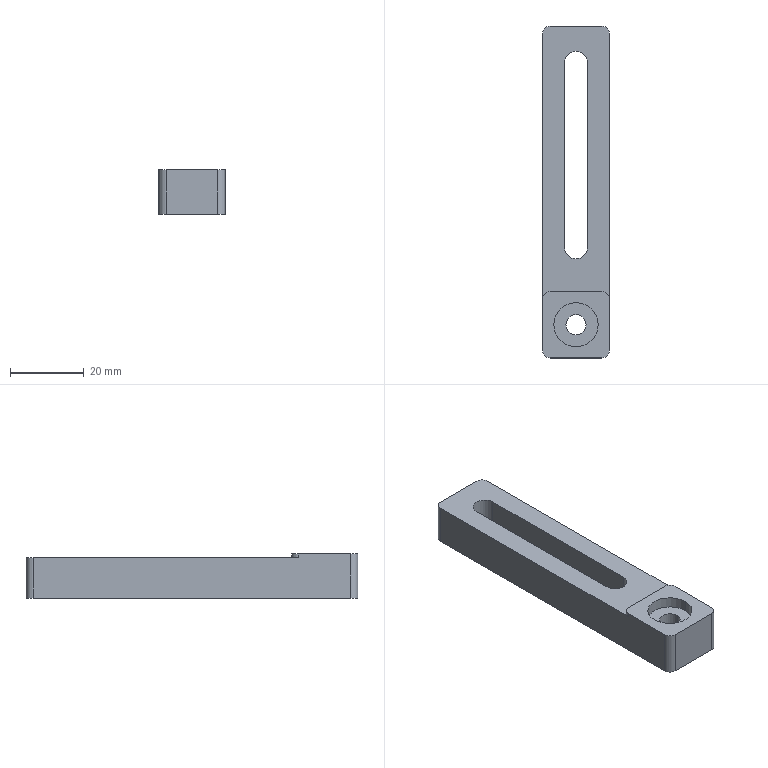Part | STEP file | 10000020588swp000-1 | 1 solid | 26 faces | box 18 x 90 x 12 mm | volume 13483 mm3 | cylinder 14 | plane 12 | commonest cylinder face diameters 4 x6 5.5 x2 6.3 x2 9.5 x2 12 x2
STEP:
#1=CARTESIAN_POINT('',(4.75,-36.,5.5));
#2=VERTEX_POINT('',#1);
#3=CARTESIAN_POINT('',(-4.75,-36.,5.5));
#4=VERTEX_POINT('',#3);
#5=CARTESIAN_POINT('',(0.,-36.,5.5));
#6=DIRECTION('',(0.,0.,-1.));
#7=DIRECTION('',(-1.,0.,0.));
#8=AXIS2_PLACEMENT_3D('',#5,#6,#7);
#9=CIRCLE('',#8,4.75);
#10=EDGE_CURVE('',#2,#4,#9,.T.);
#11=ORIENTED_EDGE('',*,*,#10,.F.);
#12=CARTESIAN_POINT('',(4.75,-36.,0.));
#13=VERTEX_POINT('',#12);
#14=CARTESIAN_POINT('',(4.75,-36.,0.));
#15=DIRECTION('',(0.,0.,-1.));
#16=VECTOR('',#15,1000.);
#17=LINE('',#14,#16);
#18=EDGE_CURVE('',#2,#13,#17,.T.);
#19=ORIENTED_EDGE('',*,*,#18,.T.);
#20=CARTESIAN_POINT('',(-4.75,-36.,0.));
#21=VERTEX_POINT('',#20);
#22=CARTESIAN_POINT('',(0.,-36.,0.));
#23=DIRECTION('',(0.,0.,-1.));
#24=DIRECTION('',(-1.,0.,0.));
#25=AXIS2_PLACEMENT_3D('',#22,#23,#24);
#26=CIRCLE('',#25,4.75);
#27=EDGE_CURVE('',#13,#21,#26,.T.);
#28=ORIENTED_EDGE('',*,*,#27,.T.);
#29=CARTESIAN_POINT('',(-4.75,-36.,0.));
#30=DIRECTION('',(0.,0.,-1.));
#31=VECTOR('',#30,1000.);
#32=LINE('',#29,#31);
#33=EDGE_CURVE('',#4,#21,#32,.T.);
#34=ORIENTED_EDGE('',*,*,#33,.F.);
#35=EDGE_LOOP('',(#11,#19,#28,#34));
#36=FACE_OUTER_BOUND('',#35,.T.);
#37=CARTESIAN_POINT('',(0.,-36.,0.));
#38=DIRECTION('',(0.,0.,-1.));
#39=DIRECTION('',(-1.,0.,0.));
#40=AXIS2_PLACEMENT_3D('',#37,#38,#39);
#41=CYLINDRICAL_SURFACE('',#40,4.75);
#42=ADVANCED_FACE('',(#36),#41,.F.);
#43=CARTESIAN_POINT('',(-6.,-36.,9.));
#44=VERTEX_POINT('',#43);
#45=CARTESIAN_POINT('',(6.,-36.,9.));
#46=VERTEX_POINT('',#45);
#47=CARTESIAN_POINT('',(0.,-36.,9.));
#48=DIRECTION('',(0.,0.,1.));
#49=DIRECTION('',(1.,0.,0.));
#50=AXIS2_PLACEMENT_3D('',#47,#48,#49);
#51=CIRCLE('',#50,6.);
#52=EDGE_CURVE('',#44,#46,#51,.T.);
#53=ORIENTED_EDGE('',*,*,#52,.F.);
#54=CARTESIAN_POINT('',(-6.,-36.,12.));
#55=VERTEX_POINT('',#54);
#56=CARTESIAN_POINT('',(-6.,-36.,12.));
#57=DIRECTION('',(0.,0.,1.));
#58=VECTOR('',#57,1000.);
#59=LINE('',#56,#58);
#60=EDGE_CURVE('',#44,#55,#59,.T.);
#61=ORIENTED_EDGE('',*,*,#60,.T.);
#62=CARTESIAN_POINT('',(6.,-36.,12.));
#63=VERTEX_POINT('',#62);
#64=CARTESIAN_POINT('',(0.,-36.,12.));
#65=DIRECTION('',(0.,0.,1.));
#66=DIRECTION('',(1.,0.,0.));
#67=AXIS2_PLACEMENT_3D('',#64,#65,#66);
#68=CIRCLE('',#67,6.);
#69=EDGE_CURVE('',#55,#63,#68,.T.);
#70=ORIENTED_EDGE('',*,*,#69,.T.);
#71=CARTESIAN_POINT('',(6.,-36.,12.));
#72=DIRECTION('',(0.,0.,1.));
#73=VECTOR('',#72,1000.);
#74=LINE('',#71,#73);
#75=EDGE_CURVE('',#46,#63,#74,.T.);
#76=ORIENTED_EDGE('',*,*,#75,.F.);
#77=EDGE_LOOP('',(#53,#61,#70,#76));
#78=FACE_OUTER_BOUND('',#77,.T.);
#79=CARTESIAN_POINT('',(0.,-36.,12.));
#80=DIRECTION('',(0.,0.,1.));
#81=DIRECTION('',(1.,0.,0.));
#82=AXIS2_PLACEMENT_3D('',#79,#80,#81);
#83=CYLINDRICAL_SURFACE('',#82,6.);
#84=ADVANCED_FACE('',(#78),#83,.F.);
#85=CARTESIAN_POINT('',(2.75,-36.,5.5));
#86=VERTEX_POINT('',#85);
#87=CARTESIAN_POINT('',(-2.75,-36.,5.5));
#88=VERTEX_POINT('',#87);
#89=CARTESIAN_POINT('',(0.,-36.,5.5));
#90=DIRECTION('',(0.,0.,-1.));
#91=DIRECTION('',(1.,0.,0.));
#92=AXIS2_PLACEMENT_3D('',#89,#90,#91);
#93=CIRCLE('',#92,2.75);
#94=EDGE_CURVE('',#86,#88,#93,.T.);
#95=ORIENTED_EDGE('',*,*,#94,.T.);
#96=CARTESIAN_POINT('',(-2.75,-36.,9.));
#97=VERTEX_POINT('',#96);
#98=CARTESIAN_POINT('',(-2.75,-36.,12.));
#99=DIRECTION('',(0.,0.,1.));
#100=VECTOR('',#99,1000.);
#101=LINE('',#98,#100);
#102=EDGE_CURVE('',#88,#97,#101,.T.);
#103=ORIENTED_EDGE('',*,*,#102,.T.);
#104=CARTESIAN_POINT('',(2.75,-36.,9.));
#105=VERTEX_POINT('',#104);
#106=CARTESIAN_POINT('',(0.,-36.,9.));
#107=DIRECTION('',(0.,0.,1.));
#108=DIRECTION('',(1.,0.,0.));
#109=AXIS2_PLACEMENT_3D('',#106,#107,#108);
#110=CIRCLE('',#109,2.75);
#111=EDGE_CURVE('',#97,#105,#110,.T.);
#112=ORIENTED_EDGE('',*,*,#111,.T.);
#113=CARTESIAN_POINT('',(2.75,-36.,12.));
#114=DIRECTION('',(0.,0.,1.));
#115=VECTOR('',#114,1000.);
#116=LINE('',#113,#115);
#117=EDGE_CURVE('',#86,#105,#116,.T.);
#118=ORIENTED_EDGE('',*,*,#117,.F.);
#119=EDGE_LOOP('',(#95,#103,#112,#118));
#120=FACE_OUTER_BOUND('',#119,.T.);
#121=CARTESIAN_POINT('',(0.,-36.,12.));
#122=DIRECTION('',(0.,0.,1.));
#123=DIRECTION('',(1.,0.,0.));
#124=AXIS2_PLACEMENT_3D('',#121,#122,#123);
#125=CYLINDRICAL_SURFACE('',#124,2.75);
#126=ADVANCED_FACE('',(#120),#125,.F.);
#127=CARTESIAN_POINT('',(7.,45.,0.));
#128=VERTEX_POINT('',#127);
#129=CARTESIAN_POINT('',(-7.,45.,0.));
#130=VERTEX_POINT('',#129);
#131=CARTESIAN_POINT('',(-9.,45.,0.));
#132=DIRECTION('',(-1.,0.,0.));
#133=VECTOR('',#132,1000.);
#134=LINE('',#131,#133);
#135=EDGE_CURVE('',#128,#130,#134,.T.);
#136=ORIENTED_EDGE('',*,*,#135,.T.);
#137=CARTESIAN_POINT('',(-7.,45.,11.));
#138=VERTEX_POINT('',#137);
#139=CARTESIAN_POINT('',(-7.,45.,12.));
#140=DIRECTION('',(0.,0.,1.));
#141=VECTOR('',#140,1000.);
#142=LINE('',#139,#141);
#143=EDGE_CURVE('',#130,#138,#142,.T.);
#144=ORIENTED_EDGE('',*,*,#143,.T.);
#145=CARTESIAN_POINT('',(7.,45.,11.));
#146=VERTEX_POINT('',#145);
#147=CARTESIAN_POINT('',(-9.,45.,11.));
#148=DIRECTION('',(-1.,0.,0.));
#149=VECTOR('',#148,1000.);
#150=LINE('',#147,#149);
#151=EDGE_CURVE('',#146,#138,#150,.T.);
#152=ORIENTED_EDGE('',*,*,#151,.F.);
#153=CARTESIAN_POINT('',(7.,45.,12.));
#154=DIRECTION('',(0.,0.,-1.));
#155=VECTOR('',#154,1000.);
#156=LINE('',#153,#155);
#157=EDGE_CURVE('',#146,#128,#156,.T.);
#158=ORIENTED_EDGE('',*,*,#157,.T.);
#159=EDGE_LOOP('',(#136,#144,#152,#158));
#160=FACE_OUTER_BOUND('',#159,.T.);
#161=CARTESIAN_POINT('',(-9.,45.,12.));
#162=DIRECTION('',(0.,-1.,0.));
#163=DIRECTION('',(0.,0.,-1.));
#164=AXIS2_PLACEMENT_3D('',#161,#162,#163);
#165=PLANE('',#164);
#166=ADVANCED_FACE('',(#160),#165,.F.);
#167=CARTESIAN_POINT('',(9.,-29.,11.));
#168=VERTEX_POINT('',#167);
#169=CARTESIAN_POINT('',(9.,43.,11.));
#170=VERTEX_POINT('',#169);
#171=CARTESIAN_POINT('',(9.,45.,11.));
#172=DIRECTION('',(0.,1.,0.));
#173=VECTOR('',#172,1000.);
#174=LINE('',#171,#173);
#175=EDGE_CURVE('',#168,#170,#174,.T.);
#176=ORIENTED_EDGE('',*,*,#175,.F.);
#177=CARTESIAN_POINT('',(9.,-29.,12.));
#178=VERTEX_POINT('',#177);
#179=CARTESIAN_POINT('',(9.,-29.,12.));
#180=DIRECTION('',(0.,0.,1.));
#181=VECTOR('',#180,1000.);
#182=LINE('',#179,#181);
#183=EDGE_CURVE('',#168,#178,#182,.T.);
#184=ORIENTED_EDGE('',*,*,#183,.T.);
#185=CARTESIAN_POINT('',(9.,-43.,12.));
#186=VERTEX_POINT('',#185);
#187=CARTESIAN_POINT('',(9.,45.,12.));
#188=DIRECTION('',(0.,1.,0.));
#189=VECTOR('',#188,1000.);
#190=LINE('',#187,#189);
#191=EDGE_CURVE('',#186,#178,#190,.T.);
#192=ORIENTED_EDGE('',*,*,#191,.F.);
#193=CARTESIAN_POINT('',(9.,-43.,0.));
#194=VERTEX_POINT('',#193);
#195=CARTESIAN_POINT('',(9.,-43.,12.));
#196=DIRECTION('',(0.,0.,-1.));
#197=VECTOR('',#196,1000.);
#198=LINE('',#195,#197);
#199=EDGE_CURVE('',#186,#194,#198,.T.);
#200=ORIENTED_EDGE('',*,*,#199,.T.);
#201=CARTESIAN_POINT('',(9.,43.,0.));
#202=VERTEX_POINT('',#201);
#203=CARTESIAN_POINT('',(9.,45.,0.));
#204=DIRECTION('',(0.,1.,0.));
#205=VECTOR('',#204,1000.);
#206=LINE('',#203,#205);
#207=EDGE_CURVE('',#194,#202,#206,.T.);
#208=ORIENTED_EDGE('',*,*,#207,.T.);
#209=CARTESIAN_POINT('',(9.,43.,12.));
#210=DIRECTION('',(0.,0.,1.));
#211=VECTOR('',#210,1000.);
#212=LINE('',#209,#211);
#213=EDGE_CURVE('',#202,#170,#212,.T.);
#214=ORIENTED_EDGE('',*,*,#213,.T.);
#215=EDGE_LOOP('',(#176,#184,#192,#200,#208,#214));
#216=FACE_OUTER_BOUND('',#215,.T.);
#217=CARTESIAN_POINT('',(9.,45.,12.));
#218=DIRECTION('',(-1.,0.,0.));
#219=DIRECTION('',(0.,-1.,0.));
#220=AXIS2_PLACEMENT_3D('',#217,#218,#219);
#221=PLANE('',#220);
#222=ADVANCED_FACE('',(#216),#221,.F.);
#223=CARTESIAN_POINT('',(-9.,-29.,12.));
#224=VERTEX_POINT('',#223);
#225=CARTESIAN_POINT('',(-9.,-43.,12.));
#226=VERTEX_POINT('',#225);
#227=CARTESIAN_POINT('',(-9.,45.,12.));
#228=DIRECTION('',(0.,-1.,0.));
#229=VECTOR('',#228,1000.);
#230=LINE('',#227,#229);
#231=EDGE_CURVE('',#224,#226,#230,.T.);
#232=ORIENTED_EDGE('',*,*,#231,.F.);
#233=CARTESIAN_POINT('',(-9.,-29.,11.));
#234=VERTEX_POINT('',#233);
#235=CARTESIAN_POINT('',(-9.,-29.,12.));
#236=DIRECTION('',(0.,0.,-1.));
#237=VECTOR('',#236,1000.);
#238=LINE('',#235,#237);
#239=EDGE_CURVE('',#224,#234,#238,.T.);
#240=ORIENTED_EDGE('',*,*,#239,.T.);
#241=CARTESIAN_POINT('',(-9.,43.,11.));
#242=VERTEX_POINT('',#241);
#243=CARTESIAN_POINT('',(-9.,45.,11.));
#244=DIRECTION('',(0.,-1.,0.));
#245=VECTOR('',#244,1000.);
#246=LINE('',#243,#245);
#247=EDGE_CURVE('',#242,#234,#246,.T.);
#248=ORIENTED_EDGE('',*,*,#247,.F.);
#249=CARTESIAN_POINT('',(-9.,43.,0.));
#250=VERTEX_POINT('',#249);
#251=CARTESIAN_POINT('',(-9.,43.,12.));
#252=DIRECTION('',(0.,0.,-1.));
#253=VECTOR('',#252,1000.);
#254=LINE('',#251,#253);
#255=EDGE_CURVE('',#242,#250,#254,.T.);
#256=ORIENTED_EDGE('',*,*,#255,.T.);
#257=CARTESIAN_POINT('',(-9.,-43.,0.));
#258=VERTEX_POINT('',#257);
#259=CARTESIAN_POINT('',(-9.,45.,0.));
#260=DIRECTION('',(0.,-1.,0.));
#261=VECTOR('',#260,1000.);
#262=LINE('',#259,#261);
#263=EDGE_CURVE('',#250,#258,#262,.T.);
#264=ORIENTED_EDGE('',*,*,#263,.T.);
#265=CARTESIAN_POINT('',(-9.,-43.,12.));
#266=DIRECTION('',(0.,0.,1.));
#267=VECTOR('',#266,1000.);
#268=LINE('',#265,#267);
#269=EDGE_CURVE('',#258,#226,#268,.T.);
#270=ORIENTED_EDGE('',*,*,#269,.T.);
#271=EDGE_LOOP('',(#232,#240,#248,#256,#264,#270));
#272=FACE_OUTER_BOUND('',#271,.T.);
#273=CARTESIAN_POINT('',(-9.,45.,12.));
#274=DIRECTION('',(1.,0.,0.));
#275=DIRECTION('',(0.,1.,0.));
#276=AXIS2_PLACEMENT_3D('',#273,#274,#275);
#277=PLANE('',#276);
#278=ADVANCED_FACE('',(#272),#277,.F.);
#279=CARTESIAN_POINT('',(-7.,-45.,0.));
#280=VERTEX_POINT('',#279);
#281=CARTESIAN_POINT('',(7.,-45.,0.));
#282=VERTEX_POINT('',#281);
#283=CARTESIAN_POINT('',(-9.,-45.,0.));
#284=DIRECTION('',(1.,0.,0.));
#285=VECTOR('',#284,1000.);
#286=LINE('',#283,#285);
#287=EDGE_CURVE('',#280,#282,#286,.T.);
#288=ORIENTED_EDGE('',*,*,#287,.T.);
#289=CARTESIAN_POINT('',(7.,-45.,12.));
#290=VERTEX_POINT('',#289);
#291=CARTESIAN_POINT('',(7.,-45.,12.));
#292=DIRECTION('',(0.,0.,1.));
#293=VECTOR('',#292,1000.);
#294=LINE('',#291,#293);
#295=EDGE_CURVE('',#282,#290,#294,.T.);
#296=ORIENTED_EDGE('',*,*,#295,.T.);
#297=CARTESIAN_POINT('',(-7.,-45.,12.));
#298=VERTEX_POINT('',#297);
#299=CARTESIAN_POINT('',(-9.,-45.,12.));
#300=DIRECTION('',(1.,0.,0.));
#301=VECTOR('',#300,1000.);
#302=LINE('',#299,#301);
#303=EDGE_CURVE('',#298,#290,#302,.T.);
#304=ORIENTED_EDGE('',*,*,#303,.F.);
#305=CARTESIAN_POINT('',(-7.,-45.,12.));
#306=DIRECTION('',(0.,0.,-1.));
#307=VECTOR('',#306,1000.);
#308=LINE('',#305,#307);
#309=EDGE_CURVE('',#298,#280,#308,.T.);
#310=ORIENTED_EDGE('',*,*,#309,.T.);
#311=EDGE_LOOP('',(#288,#296,#304,#310));
#312=FACE_OUTER_BOUND('',#311,.T.);
#313=CARTESIAN_POINT('',(-9.,-45.,12.));
#314=DIRECTION('',(0.,1.,0.));
#315=DIRECTION('',(0.,0.,1.));
#316=AXIS2_PLACEMENT_3D('',#313,#314,#315);
#317=PLANE('',#316);
#318=ADVANCED_FACE('',(#312),#317,.F.);
#319=CARTESIAN_POINT('',(0.,-36.,12.));
#320=DIRECTION('',(0.,0.,1.));
#321=DIRECTION('',(1.,0.,0.));
#322=AXIS2_PLACEMENT_3D('',#319,#320,#321);
#323=CIRCLE('',#322,6.);
#324=EDGE_CURVE('',#63,#55,#323,.T.);
#325=ORIENTED_EDGE('',*,*,#324,.F.);
#326=ORIENTED_EDGE('',*,*,#69,.F.);
#327=EDGE_LOOP('',(#325,#326));
#328=FACE_BOUND('',#327,.T.);
#329=CARTESIAN_POINT('',(-7.,-27.,12.));
#330=VERTEX_POINT('',#329);
#331=CARTESIAN_POINT('',(7.,-27.,12.));
#332=VERTEX_POINT('',#331);
#333=CARTESIAN_POINT('',(-9.,-27.,12.));
#334=DIRECTION('',(1.,0.,0.));
#335=VECTOR('',#334,1000.);
#336=LINE('',#333,#335);
#337=EDGE_CURVE('',#330,#332,#336,.T.);
#338=ORIENTED_EDGE('',*,*,#337,.F.);
#339=CARTESIAN_POINT('',(-7.,-29.,12.));
#340=DIRECTION('',(0.,0.,1.));
#341=DIRECTION('',(1.,0.,0.));
#342=AXIS2_PLACEMENT_3D('',#339,#340,#341);
#343=CIRCLE('',#342,2.);
#344=EDGE_CURVE('',#330,#224,#343,.T.);
#345=ORIENTED_EDGE('',*,*,#344,.T.);
#346=ORIENTED_EDGE('',*,*,#231,.T.);
#347=CARTESIAN_POINT('',(-7.,-43.,12.));
#348=DIRECTION('',(0.,0.,1.));
#349=DIRECTION('',(1.,0.,0.));
#350=AXIS2_PLACEMENT_3D('',#347,#348,#349);
#351=CIRCLE('',#350,2.);
#352=EDGE_CURVE('',#226,#298,#351,.T.);
#353=ORIENTED_EDGE('',*,*,#352,.T.);
#354=ORIENTED_EDGE('',*,*,#303,.T.);
#355=CARTESIAN_POINT('',(7.,-43.,12.));
#356=DIRECTION('',(0.,0.,1.));
#357=DIRECTION('',(1.,0.,0.));
#358=AXIS2_PLACEMENT_3D('',#355,#356,#357);
#359=CIRCLE('',#358,2.);
#360=EDGE_CURVE('',#290,#186,#359,.T.);
#361=ORIENTED_EDGE('',*,*,#360,.T.);
#362=ORIENTED_EDGE('',*,*,#191,.T.);
#363=CARTESIAN_POINT('',(7.,-29.,12.));
#364=DIRECTION('',(0.,0.,1.));
#365=DIRECTION('',(1.,0.,0.));
#366=AXIS2_PLACEMENT_3D('',#363,#364,#365);
#367=CIRCLE('',#366,2.);
#368=EDGE_CURVE('',#178,#332,#367,.T.);
#369=ORIENTED_EDGE('',*,*,#368,.T.);
#370=EDGE_LOOP('',(#338,#345,#346,#353,#354,#361,#362,#369));
#371=FACE_OUTER_BOUND('',#370,.T.);
#372=CARTESIAN_POINT('',(0.,0.,12.));
#373=DIRECTION('',(0.,0.,1.));
#374=DIRECTION('',(1.,0.,0.));
#375=AXIS2_PLACEMENT_3D('',#372,#373,#374);
#376=PLANE('',#375);
#377=ADVANCED_FACE('',(#328,#371),#376,.T.);
#378=CARTESIAN_POINT('',(0.,-36.,0.));
#379=DIRECTION('',(0.,0.,-1.));
#380=DIRECTION('',(-1.,0.,0.));
#381=AXIS2_PLACEMENT_3D('',#378,#379,#380);
#382=CIRCLE('',#381,4.75);
#383=EDGE_CURVE('',#21,#13,#382,.T.);
#384=ORIENTED_EDGE('',*,*,#383,.F.);
#385=ORIENTED_EDGE('',*,*,#27,.F.);
#386=EDGE_LOOP('',(#384,#385));
#387=FACE_BOUND('',#386,.T.);
#388=CARTESIAN_POINT('',(3.15,-15.,0.));
#389=VERTEX_POINT('',#388);
#390=CARTESIAN_POINT('',(3.15,35.,0.));
#391=VERTEX_POINT('',#390);
#392=CARTESIAN_POINT('',(3.15,35.,0.));
#393=DIRECTION('',(0.,1.,0.));
#394=VECTOR('',#393,1000.);
#395=LINE('',#392,#394);
#396=EDGE_CURVE('',#389,#391,#395,.T.);
#397=ORIENTED_EDGE('',*,*,#396,.T.);
#398=CARTESIAN_POINT('',(-3.15,35.,0.));
#399=VERTEX_POINT('',#398);
#400=CARTESIAN_POINT('',(0.,35.,0.));
#401=DIRECTION('',(0.,0.,1.));
#402=DIRECTION('',(1.,0.,0.));
#403=AXIS2_PLACEMENT_3D('',#400,#401,#402);
#404=CIRCLE('',#403,3.15);
#405=EDGE_CURVE('',#391,#399,#404,.T.);
#406=ORIENTED_EDGE('',*,*,#405,.T.);
#407=CARTESIAN_POINT('',(-3.15,-15.,0.));
#408=VERTEX_POINT('',#407);
#409=CARTESIAN_POINT('',(-3.15,35.,0.));
#410=DIRECTION('',(0.,-1.,0.));
#411=VECTOR('',#410,1000.);
#412=LINE('',#409,#411);
#413=EDGE_CURVE('',#399,#408,#412,.T.);
#414=ORIENTED_EDGE('',*,*,#413,.T.);
#415=CARTESIAN_POINT('',(0.,-15.,0.));
#416=DIRECTION('',(0.,0.,1.));
#417=DIRECTION('',(1.,0.,0.));
#418=AXIS2_PLACEMENT_3D('',#415,#416,#417);
#419=CIRCLE('',#418,3.15);
#420=EDGE_CURVE('',#408,#389,#419,.T.);
#421=ORIENTED_EDGE('',*,*,#420,.T.);
#422=EDGE_LOOP('',(#397,#406,#414,#421));
#423=FACE_BOUND('',#422,.T.);
#424=ORIENTED_EDGE('',*,*,#207,.F.);
#425=CARTESIAN_POINT('',(7.,-43.,0.));
#426=DIRECTION('',(0.,0.,-1.));
#427=DIRECTION('',(1.,0.,0.));
#428=AXIS2_PLACEMENT_3D('',#425,#426,#427);
#429=CIRCLE('',#428,2.);
#430=EDGE_CURVE('',#194,#282,#429,.T.);
#431=ORIENTED_EDGE('',*,*,#430,.T.);
#432=ORIENTED_EDGE('',*,*,#287,.F.);
#433=CARTESIAN_POINT('',(-7.,-43.,0.));
#434=DIRECTION('',(0.,0.,-1.));
#435=DIRECTION('',(1.,0.,0.));
#436=AXIS2_PLACEMENT_3D('',#433,#434,#435);
#437=CIRCLE('',#436,2.);
#438=EDGE_CURVE('',#280,#258,#437,.T.);
#439=ORIENTED_EDGE('',*,*,#438,.T.);
#440=ORIENTED_EDGE('',*,*,#263,.F.);
#441=CARTESIAN_POINT('',(-7.,43.,0.));
#442=DIRECTION('',(0.,0.,-1.));
#443=DIRECTION('',(1.,0.,0.));
#444=AXIS2_PLACEMENT_3D('',#441,#442,#443);
#445=CIRCLE('',#444,2.);
#446=EDGE_CURVE('',#250,#130,#445,.T.);
#447=ORIENTED_EDGE('',*,*,#446,.T.);
#448=ORIENTED_EDGE('',*,*,#135,.F.);
#449=CARTESIAN_POINT('',(7.,43.,0.));
#450=DIRECTION('',(0.,0.,-1.));
#451=DIRECTION('',(1.,0.,0.));
#452=AXIS2_PLACEMENT_3D('',#449,#450,#451);
#453=CIRCLE('',#452,2.);
#454=EDGE_CURVE('',#128,#202,#453,.T.);
#455=ORIENTED_EDGE('',*,*,#454,.T.);
#456=EDGE_LOOP('',(#424,#431,#432,#439,#440,#447,#448,#455));
#457=FACE_OUTER_BOUND('',#456,.T.);
#458=CARTESIAN_POINT('',(0.,0.,0.));
#459=DIRECTION('',(0.,0.,1.));
#460=DIRECTION('',(1.,0.,0.));
#461=AXIS2_PLACEMENT_3D('',#458,#459,#460);
#462=PLANE('',#461);
#463=ADVANCED_FACE('',(#387,#423,#457),#462,.F.);
#464=CARTESIAN_POINT('',(-7.,-27.,11.));
#465=VERTEX_POINT('',#464);
#466=CARTESIAN_POINT('',(7.,-27.,11.));
#467=VERTEX_POINT('',#466);
#468=CARTESIAN_POINT('',(-9.,-27.,11.));
#469=DIRECTION('',(1.,0.,0.));
#470=VECTOR('',#469,1000.);
#471=LINE('',#468,#470);
#472=EDGE_CURVE('',#465,#467,#471,.T.);
#473=ORIENTED_EDGE('',*,*,#472,.F.);
#474=CARTESIAN_POINT('',(-7.,-27.,11.));
#475=DIRECTION('',(0.,0.,1.));
#476=VECTOR('',#475,1000.);
#477=LINE('',#474,#476);
#478=EDGE_CURVE('',#465,#330,#477,.T.);
#479=ORIENTED_EDGE('',*,*,#478,.T.);
#480=ORIENTED_EDGE('',*,*,#337,.T.);
#481=CARTESIAN_POINT('',(7.,-27.,11.));
#482=DIRECTION('',(0.,0.,-1.));
#483=VECTOR('',#482,1000.);
#484=LINE('',#481,#483);
#485=EDGE_CURVE('',#332,#467,#484,.T.);
#486=ORIENTED_EDGE('',*,*,#485,.T.);
#487=EDGE_LOOP('',(#473,#479,#480,#486));
#488=FACE_OUTER_BOUND('',#487,.T.);
#489=CARTESIAN_POINT('',(-9.,-27.,11.));
#490=DIRECTION('',(0.,-1.,0.));
#491=DIRECTION('',(0.,0.,-1.));
#492=AXIS2_PLACEMENT_3D('',#489,#490,#491);
#493=PLANE('',#492);
#494=ADVANCED_FACE('',(#488),#493,.F.);
#495=CARTESIAN_POINT('',(3.15,35.,11.));
#496=VERTEX_POINT('',#495);
#497=CARTESIAN_POINT('',(-3.15,35.,11.));
#498=VERTEX_POINT('',#497);
#499=CARTESIAN_POINT('',(0.,35.,11.));
#500=DIRECTION('',(0.,0.,1.));
#501=DIRECTION('',(1.,0.,0.));
#502=AXIS2_PLACEMENT_3D('',#499,#500,#501);
#503=CIRCLE('',#502,3.15);
#504=EDGE_CURVE('',#496,#498,#503,.T.);
#505=ORIENTED_EDGE('',*,*,#504,.F.);
#506=CARTESIAN_POINT('',(3.15,-15.,11.));
#507=VERTEX_POINT('',#506);
#508=CARTESIAN_POINT('',(3.15,0.,11.));
#509=DIRECTION('',(0.,1.,0.));
#510=VECTOR('',#509,1000.);
#511=LINE('',#508,#510);
#512=EDGE_CURVE('',#507,#496,#511,.T.);
#513=ORIENTED_EDGE('',*,*,#512,.F.);
#514=CARTESIAN_POINT('',(-3.15,-15.,11.));
#515=VERTEX_POINT('',#514);
#516=CARTESIAN_POINT('',(0.,-15.,11.));
#517=DIRECTION('',(0.,0.,1.));
#518=DIRECTION('',(1.,0.,0.));
#519=AXIS2_PLACEMENT_3D('',#516,#517,#518);
#520=CIRCLE('',#519,3.15);
#521=EDGE_CURVE('',#515,#507,#520,.T.);
#522=ORIENTED_EDGE('',*,*,#521,.F.);
#523=CARTESIAN_POINT('',(-3.15,0.,11.));
#524=DIRECTION('',(0.,-1.,0.));
#525=VECTOR('',#524,1000.);
#526=LINE('',#523,#525);
#527=EDGE_CURVE('',#498,#515,#526,.T.);
#528=ORIENTED_EDGE('',*,*,#527,.F.);
#529=EDGE_LOOP('',(#505,#513,#522,#528));
#530=FACE_BOUND('',#529,.T.);
#531=ORIENTED_EDGE('',*,*,#151,.T.);
#532=CARTESIAN_POINT('',(-7.,43.,11.));
#533=DIRECTION('',(0.,0.,1.));
#534=DIRECTION('',(1.,0.,0.));
#535=AXIS2_PLACEMENT_3D('',#532,#533,#534);
#536=CIRCLE('',#535,2.);
#537=EDGE_CURVE('',#138,#242,#536,.T.);
#538=ORIENTED_EDGE('',*,*,#537,.T.);
#539=ORIENTED_EDGE('',*,*,#247,.T.);
#540=CARTESIAN_POINT('',(-7.,-29.,11.));
#541=DIRECTION('',(0.,0.,-1.));
#542=DIRECTION('',(1.,0.,0.));
#543=AXIS2_PLACEMENT_3D('',#540,#541,#542);
#544=CIRCLE('',#543,2.);
#545=EDGE_CURVE('',#234,#465,#544,.T.);
#546=ORIENTED_EDGE('',*,*,#545,.T.);
#547=ORIENTED_EDGE('',*,*,#472,.T.);
#548=CARTESIAN_POINT('',(7.,-29.,11.));
#549=DIRECTION('',(0.,0.,-1.));
#550=DIRECTION('',(1.,0.,0.));
#551=AXIS2_PLACEMENT_3D('',#548,#549,#550);
#552=CIRCLE('',#551,2.);
#553=EDGE_CURVE('',#467,#168,#552,.T.);
#554=ORIENTED_EDGE('',*,*,#553,.T.);
#555=ORIENTED_EDGE('',*,*,#175,.T.);
#556=CARTESIAN_POINT('',(7.,43.,11.));
#557=DIRECTION('',(0.,0.,1.));
#558=DIRECTION('',(1.,0.,0.));
#559=AXIS2_PLACEMENT_3D('',#556,#557,#558);
#560=CIRCLE('',#559,2.);
#561=EDGE_CURVE('',#170,#146,#560,.T.);
#562=ORIENTED_EDGE('',*,*,#561,.T.);
#563=EDGE_LOOP('',(#531,#538,#539,#546,#547,#554,#555,#562));
#564=FACE_OUTER_BOUND('',#563,.T.);
#565=CARTESIAN_POINT('',(0.,0.,11.));
#566=DIRECTION('',(0.,0.,1.));
#567=DIRECTION('',(1.,0.,0.));
#568=AXIS2_PLACEMENT_3D('',#565,#566,#567);
#569=PLANE('',#568);
#570=ADVANCED_FACE('',(#530,#564),#569,.T.);
#571=ORIENTED_EDGE('',*,*,#504,.T.);
#572=CARTESIAN_POINT('',(-3.15,35.,0.));
#573=DIRECTION('',(0.,0.,1.));
#574=VECTOR('',#573,1000.);
#575=LINE('',#572,#574);
#576=EDGE_CURVE('',#399,#498,#575,.T.);
#577=ORIENTED_EDGE('',*,*,#576,.F.);
#578=ORIENTED_EDGE('',*,*,#405,.F.);
#579=CARTESIAN_POINT('',(3.15,35.,0.));
#580=DIRECTION('',(0.,0.,1.));
#581=VECTOR('',#580,1000.);
#582=LINE('',#579,#581);
#583=EDGE_CURVE('',#391,#496,#582,.T.);
#584=ORIENTED_EDGE('',*,*,#583,.T.);
#585=EDGE_LOOP('',(#571,#577,#578,#584));
#586=FACE_OUTER_BOUND('',#585,.T.);
#587=CARTESIAN_POINT('',(0.,35.,0.));
#588=DIRECTION('',(0.,0.,1.));
#589=DIRECTION('',(1.,0.,0.));
#590=AXIS2_PLACEMENT_3D('',#587,#588,#589);
#591=CYLINDRICAL_SURFACE('',#590,3.15);
#592=ADVANCED_FACE('',(#586),#591,.F.);
#593=ORIENTED_EDGE('',*,*,#512,.T.);
#594=ORIENTED_EDGE('',*,*,#583,.F.);
#595=ORIENTED_EDGE('',*,*,#396,.F.);
#596=CARTESIAN_POINT('',(3.15,-15.,0.));
#597=DIRECTION('',(0.,0.,1.));
#598=VECTOR('',#597,1000.);
#599=LINE('',#596,#598);
#600=EDGE_CURVE('',#389,#507,#599,.T.);
#601=ORIENTED_EDGE('',*,*,#600,.T.);
#602=EDGE_LOOP('',(#593,#594,#595,#601));
#603=FACE_OUTER_BOUND('',#602,.T.);
#604=CARTESIAN_POINT('',(3.15,35.,0.));
#605=DIRECTION('',(1.,0.,0.));
#606=DIRECTION('',(0.,1.,0.));
#607=AXIS2_PLACEMENT_3D('',#604,#605,#606);
#608=PLANE('',#607);
#609=ADVANCED_FACE('',(#603),#608,.F.);
#610=ORIENTED_EDGE('',*,*,#521,.T.);
#611=ORIENTED_EDGE('',*,*,#600,.F.);
#612=ORIENTED_EDGE('',*,*,#420,.F.);
#613=CARTESIAN_POINT('',(-3.15,-15.,0.));
#614=DIRECTION('',(0.,0.,1.));
#615=VECTOR('',#614,1000.);
#616=LINE('',#613,#615);
#617=EDGE_CURVE('',#408,#515,#616,.T.);
#618=ORIENTED_EDGE('',*,*,#617,.T.);
#619=EDGE_LOOP('',(#610,#611,#612,#618));
#620=FACE_OUTER_BOUND('',#619,.T.);
#621=CARTESIAN_POINT('',(0.,-15.,0.));
#622=DIRECTION('',(0.,0.,1.));
#623=DIRECTION('',(1.,0.,0.));
#624=AXIS2_PLACEMENT_3D('',#621,#622,#623);
#625=CYLINDRICAL_SURFACE('',#624,3.15);
#626=ADVANCED_FACE('',(#620),#625,.F.);
#627=ORIENTED_EDGE('',*,*,#527,.T.);
#628=ORIENTED_EDGE('',*,*,#617,.F.);
#629=ORIENTED_EDGE('',*,*,#413,.F.);
#630=ORIENTED_EDGE('',*,*,#576,.T.);
#631=EDGE_LOOP('',(#627,#628,#629,#630));
#632=FACE_OUTER_BOUND('',#631,.T.);
#633=CARTESIAN_POINT('',(-3.15,35.,0.));
#634=DIRECTION('',(-1.,0.,0.));
#635=DIRECTION('',(0.,-1.,0.));
#636=AXIS2_PLACEMENT_3D('',#633,#634,#635);
#637=PLANE('',#636);
#638=ADVANCED_FACE('',(#632),#637,.F.);
#639=ORIENTED_EDGE('',*,*,#102,.F.);
#640=CARTESIAN_POINT('',(0.,-36.,5.5));
#641=DIRECTION('',(0.,0.,-1.));
#642=DIRECTION('',(1.,0.,0.));
#643=AXIS2_PLACEMENT_3D('',#640,#641,#642);
#644=CIRCLE('',#643,2.75);
#645=EDGE_CURVE('',#88,#86,#644,.T.);
#646=ORIENTED_EDGE('',*,*,#645,.T.);
#647=ORIENTED_EDGE('',*,*,#117,.T.);
#648=CARTESIAN_POINT('',(0.,-36.,9.));
#649=DIRECTION('',(0.,0.,1.));
#650=DIRECTION('',(1.,0.,0.));
#651=AXIS2_PLACEMENT_3D('',#648,#649,#650);
#652=CIRCLE('',#651,2.75);
#653=EDGE_CURVE('',#105,#97,#652,.T.);
#654=ORIENTED_EDGE('',*,*,#653,.T.);
#655=EDGE_LOOP('',(#639,#646,#647,#654));
#656=FACE_OUTER_BOUND('',#655,.T.);
#657=CARTESIAN_POINT('',(0.,-36.,12.));
#658=DIRECTION('',(0.,0.,1.));
#659=DIRECTION('',(1.,0.,0.));
#660=AXIS2_PLACEMENT_3D('',#657,#658,#659);
#661=CYLINDRICAL_SURFACE('',#660,2.75);
#662=ADVANCED_FACE('',(#656),#661,.F.);
#663=ORIENTED_EDGE('',*,*,#653,.F.);
#664=ORIENTED_EDGE('',*,*,#111,.F.);
#665=EDGE_LOOP('',(#663,#664));
#666=FACE_BOUND('',#665,.T.);
#667=CARTESIAN_POINT('',(0.,-36.,9.));
#668=DIRECTION('',(0.,0.,1.));
#669=DIRECTION('',(1.,0.,0.));
#670=AXIS2_PLACEMENT_3D('',#667,#668,#669);
#671=CIRCLE('',#670,6.);
#672=EDGE_CURVE('',#46,#44,#671,.T.);
#673=ORIENTED_EDGE('',*,*,#672,.T.);
#674=ORIENTED_EDGE('',*,*,#52,.T.);
#675=EDGE_LOOP('',(#673,#674));
#676=FACE_OUTER_BOUND('',#675,.T.);
#677=CARTESIAN_POINT('',(2.75,-36.,9.));
#678=DIRECTION('',(0.,0.,-1.));
#679=DIRECTION('',(-1.,0.,0.));
#680=AXIS2_PLACEMENT_3D('',#677,#678,#679);
#681=PLANE('',#680);
#682=ADVANCED_FACE('',(#666,#676),#681,.F.);
#683=ORIENTED_EDGE('',*,*,#60,.F.);
#684=ORIENTED_EDGE('',*,*,#672,.F.);
#685=ORIENTED_EDGE('',*,*,#75,.T.);
#686=ORIENTED_EDGE('',*,*,#324,.T.);
#687=EDGE_LOOP('',(#683,#684,#685,#686));
#688=FACE_OUTER_BOUND('',#687,.T.);
#689=CARTESIAN_POINT('',(0.,-36.,12.));
#690=DIRECTION('',(0.,0.,1.));
#691=DIRECTION('',(1.,0.,0.));
#692=AXIS2_PLACEMENT_3D('',#689,#690,#691);
#693=CYLINDRICAL_SURFACE('',#692,6.);
#694=ADVANCED_FACE('',(#688),#693,.F.);
#695=CARTESIAN_POINT('',(0.,-36.,5.5));
#696=DIRECTION('',(0.,0.,-1.));
#697=DIRECTION('',(-1.,0.,0.));
#698=AXIS2_PLACEMENT_3D('',#695,#696,#697);
#699=CIRCLE('',#698,4.75);
#700=EDGE_CURVE('',#4,#2,#699,.T.);
#701=ORIENTED_EDGE('',*,*,#700,.T.);
#702=ORIENTED_EDGE('',*,*,#10,.T.);
#703=EDGE_LOOP('',(#701,#702));
#704=FACE_OUTER_BOUND('',#703,.T.);
#705=ORIENTED_EDGE('',*,*,#94,.F.);
#706=ORIENTED_EDGE('',*,*,#645,.F.);
#707=EDGE_LOOP('',(#705,#706));
#708=FACE_BOUND('',#707,.T.);
#709=CARTESIAN_POINT('',(0.,-36.,5.5));
#710=DIRECTION('',(0.,0.,1.));
#711=DIRECTION('',(1.,0.,0.));
#712=AXIS2_PLACEMENT_3D('',#709,#710,#711);
#713=PLANE('',#712);
#714=ADVANCED_FACE('',(#704,#708),#713,.F.);
#715=ORIENTED_EDGE('',*,*,#18,.F.);
#716=ORIENTED_EDGE('',*,*,#700,.F.);
#717=ORIENTED_EDGE('',*,*,#33,.T.);
#718=ORIENTED_EDGE('',*,*,#383,.T.);
#719=EDGE_LOOP('',(#715,#716,#717,#718));
#720=FACE_OUTER_BOUND('',#719,.T.);
#721=CARTESIAN_POINT('',(0.,-36.,0.));
#722=DIRECTION('',(0.,0.,-1.));
#723=DIRECTION('',(-1.,0.,0.));
#724=AXIS2_PLACEMENT_3D('',#721,#722,#723);
#725=CYLINDRICAL_SURFACE('',#724,4.75);
#726=ADVANCED_FACE('',(#720),#725,.F.);
#727=ORIENTED_EDGE('',*,*,#360,.F.);
#728=ORIENTED_EDGE('',*,*,#295,.F.);
#729=ORIENTED_EDGE('',*,*,#430,.F.);
#730=ORIENTED_EDGE('',*,*,#199,.F.);
#731=EDGE_LOOP('',(#727,#728,#729,#730));
#732=FACE_OUTER_BOUND('',#731,.T.);
#733=CARTESIAN_POINT('',(7.,-43.,12.));
#734=DIRECTION('',(0.,0.,-1.));
#735=DIRECTION('',(-1.,0.,0.));
#736=AXIS2_PLACEMENT_3D('',#733,#734,#735);
#737=CYLINDRICAL_SURFACE('',#736,2.);
#738=ADVANCED_FACE('',(#732),#737,.T.);
#739=ORIENTED_EDGE('',*,*,#352,.F.);
#740=ORIENTED_EDGE('',*,*,#269,.F.);
#741=ORIENTED_EDGE('',*,*,#438,.F.);
#742=ORIENTED_EDGE('',*,*,#309,.F.);
#743=EDGE_LOOP('',(#739,#740,#741,#742));
#744=FACE_OUTER_BOUND('',#743,.T.);
#745=CARTESIAN_POINT('',(-7.,-43.,12.));
#746=DIRECTION('',(0.,0.,-1.));
#747=DIRECTION('',(-1.,0.,0.));
#748=AXIS2_PLACEMENT_3D('',#745,#746,#747);
#749=CYLINDRICAL_SURFACE('',#748,2.);
#750=ADVANCED_FACE('',(#744),#749,.T.);
#751=ORIENTED_EDGE('',*,*,#537,.F.);
#752=ORIENTED_EDGE('',*,*,#143,.F.);
#753=ORIENTED_EDGE('',*,*,#446,.F.);
#754=ORIENTED_EDGE('',*,*,#255,.F.);
#755=EDGE_LOOP('',(#751,#752,#753,#754));
#756=FACE_OUTER_BOUND('',#755,.T.);
#757=CARTESIAN_POINT('',(-7.,43.,12.));
#758=DIRECTION('',(0.,0.,-1.));
#759=DIRECTION('',(-1.,0.,0.));
#760=AXIS2_PLACEMENT_3D('',#757,#758,#759);
#761=CYLINDRICAL_SURFACE('',#760,2.);
#762=ADVANCED_FACE('',(#756),#761,.T.);
#763=ORIENTED_EDGE('',*,*,#561,.F.);
#764=ORIENTED_EDGE('',*,*,#213,.F.);
#765=ORIENTED_EDGE('',*,*,#454,.F.);
#766=ORIENTED_EDGE('',*,*,#157,.F.);
#767=EDGE_LOOP('',(#763,#764,#765,#766));
#768=FACE_OUTER_BOUND('',#767,.T.);
#769=CARTESIAN_POINT('',(7.,43.,12.));
#770=DIRECTION('',(0.,0.,-1.));
#771=DIRECTION('',(-1.,0.,0.));
#772=AXIS2_PLACEMENT_3D('',#769,#770,#771);
#773=CYLINDRICAL_SURFACE('',#772,2.);
#774=ADVANCED_FACE('',(#768),#773,.T.);
#775=ORIENTED_EDGE('',*,*,#545,.F.);
#776=ORIENTED_EDGE('',*,*,#239,.F.);
#777=ORIENTED_EDGE('',*,*,#344,.F.);
#778=ORIENTED_EDGE('',*,*,#478,.F.);
#779=EDGE_LOOP('',(#775,#776,#777,#778));
#780=FACE_OUTER_BOUND('',#779,.T.);
#781=CARTESIAN_POINT('',(-7.,-29.,11.));
#782=DIRECTION('',(0.,0.,1.));
#783=DIRECTION('',(1.,0.,0.));
#784=AXIS2_PLACEMENT_3D('',#781,#782,#783);
#785=CYLINDRICAL_SURFACE('',#784,2.);
#786=ADVANCED_FACE('',(#780),#785,.T.);
#787=ORIENTED_EDGE('',*,*,#553,.F.);
#788=ORIENTED_EDGE('',*,*,#485,.F.);
#789=ORIENTED_EDGE('',*,*,#368,.F.);
#790=ORIENTED_EDGE('',*,*,#183,.F.);
#791=EDGE_LOOP('',(#787,#788,#789,#790));
#792=FACE_OUTER_BOUND('',#791,.T.);
#793=CARTESIAN_POINT('',(7.,-29.,12.));
#794=DIRECTION('',(0.,0.,1.));
#795=DIRECTION('',(1.,0.,0.));
#796=AXIS2_PLACEMENT_3D('',#793,#794,#795);
#797=CYLINDRICAL_SURFACE('',#796,2.);
#798=ADVANCED_FACE('',(#792),#797,.T.);
#799=CLOSED_SHELL('',(#42,#84,#126,#166,#222,#278,#318,#377,#463,#494,#570,#592,#609,#626,#638,#662,#682,#694,#714,#726,#738,#750,#762,#774,#786,#798));
#800=MANIFOLD_SOLID_BREP('',#799);
#801=CARTESIAN_POINT('',(0.,0.,0.));
#802=DIRECTION('',(0.,0.,1.));
#803=DIRECTION('',(1.,0.,0.));
#804=AXIS2_PLACEMENT_3D('',#801,#802,#803);
#805=(LENGTH_UNIT()NAMED_UNIT(*)SI_UNIT(.MILLI.,.METRE.));
#806=UNCERTAINTY_MEASURE_WITH_UNIT(LENGTH_MEASURE(0.00001),#805,'','');
#807=(NAMED_UNIT(*)PLANE_ANGLE_UNIT()SI_UNIT($,.RADIAN.));
#808=(NAMED_UNIT(*)SI_UNIT($,.STERADIAN.)SOLID_ANGLE_UNIT());
#809=(GEOMETRIC_REPRESENTATION_CONTEXT(3)GLOBAL_UNCERTAINTY_ASSIGNED_CONTEXT((#806))GLOBAL_UNIT_ASSIGNED_CONTEXT((#805,#807,#808))REPRESENTATION_CONTEXT('',''));
#810=ADVANCED_BREP_SHAPE_REPRESENTATION('',(#800,#804),#809);